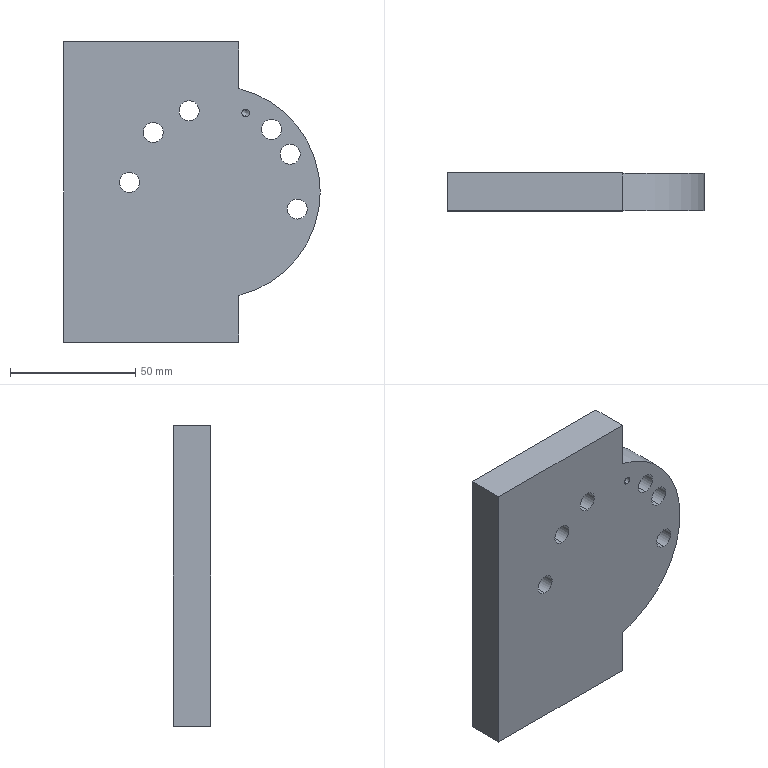Part | STEP file | jjjj_Default | 1 solid | 69 faces | box 102.5 x 15 x 120 mm | volume 138148 mm3 | cylinder 42 | plane 25 | cone 2 | commonest cylinder face diameters 12 x18 8 x12 11 x9 3 x2 85 x1